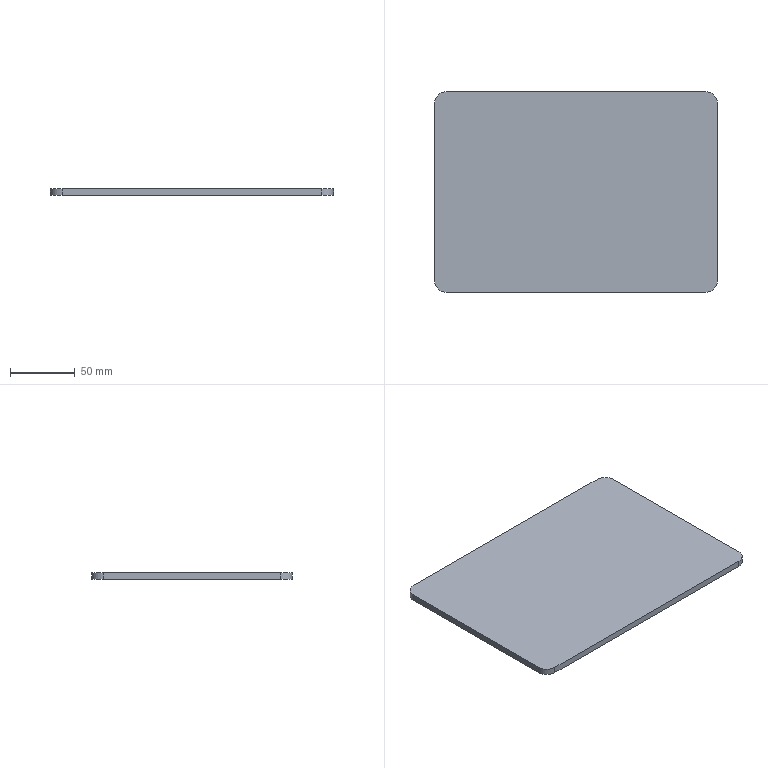Part | SolidWorks | features Extrusion 1, Fillet 1 | 1 solid | 10 faces | box 219 x 155 x 5 mm | volume 169377 mm3 | plane 6 | cylinder 4 | commonest cylinder face diameters 18 x4
STEP:
#1=CARTESIAN_POINT('',(0.,-9.,0.));
#2=VERTEX_POINT('',#1);
#3=CARTESIAN_POINT('',(0.,-146.,0.));
#4=VERTEX_POINT('',#3);
#5=CARTESIAN_POINT('',(0.,0.,0.));
#6=DIRECTION('',(0.,-1.,0.));
#7=VECTOR('',#6,1000.);
#8=LINE('',#5,#7);
#9=EDGE_CURVE('',#2,#4,#8,.T.);
#10=ORIENTED_EDGE('',*,*,#9,.T.);
#11=CARTESIAN_POINT('',(0.,-146.,5.));
#12=VERTEX_POINT('',#11);
#13=CARTESIAN_POINT('',(0.,-146.,5.));
#14=DIRECTION('',(0.,0.,1.));
#15=VECTOR('',#14,1000.);
#16=LINE('',#13,#15);
#17=EDGE_CURVE('',#4,#12,#16,.T.);
#18=ORIENTED_EDGE('',*,*,#17,.T.);
#19=CARTESIAN_POINT('',(0.,-9.,5.));
#20=VERTEX_POINT('',#19);
#21=CARTESIAN_POINT('',(0.,0.,5.));
#22=DIRECTION('',(0.,-1.,0.));
#23=VECTOR('',#22,1000.);
#24=LINE('',#21,#23);
#25=EDGE_CURVE('',#20,#12,#24,.T.);
#26=ORIENTED_EDGE('',*,*,#25,.F.);
#27=CARTESIAN_POINT('',(0.,-9.,5.));
#28=DIRECTION('',(0.,0.,-1.));
#29=VECTOR('',#28,1000.);
#30=LINE('',#27,#29);
#31=EDGE_CURVE('',#20,#2,#30,.T.);
#32=ORIENTED_EDGE('',*,*,#31,.T.);
#33=EDGE_LOOP('',(#10,#18,#26,#32));
#34=FACE_OUTER_BOUND('',#33,.T.);
#35=CARTESIAN_POINT('',(0.,0.,5.));
#36=DIRECTION('',(1.,0.,0.));
#37=DIRECTION('',(0.,1.,0.));
#38=AXIS2_PLACEMENT_3D('',#35,#36,#37);
#39=PLANE('',#38);
#40=ADVANCED_FACE('',(#34),#39,.F.);
#41=CARTESIAN_POINT('',(9.,-155.,0.));
#42=VERTEX_POINT('',#41);
#43=CARTESIAN_POINT('',(210.,-155.,0.));
#44=VERTEX_POINT('',#43);
#45=CARTESIAN_POINT('',(0.,-155.,0.));
#46=DIRECTION('',(1.,0.,0.));
#47=VECTOR('',#46,1000.);
#48=LINE('',#45,#47);
#49=EDGE_CURVE('',#42,#44,#48,.T.);
#50=ORIENTED_EDGE('',*,*,#49,.T.);
#51=CARTESIAN_POINT('',(210.,-155.,5.));
#52=VERTEX_POINT('',#51);
#53=CARTESIAN_POINT('',(210.,-155.,5.));
#54=DIRECTION('',(0.,0.,1.));
#55=VECTOR('',#54,1000.);
#56=LINE('',#53,#55);
#57=EDGE_CURVE('',#44,#52,#56,.T.);
#58=ORIENTED_EDGE('',*,*,#57,.T.);
#59=CARTESIAN_POINT('',(9.,-155.,5.));
#60=VERTEX_POINT('',#59);
#61=CARTESIAN_POINT('',(0.,-155.,5.));
#62=DIRECTION('',(1.,0.,0.));
#63=VECTOR('',#62,1000.);
#64=LINE('',#61,#63);
#65=EDGE_CURVE('',#60,#52,#64,.T.);
#66=ORIENTED_EDGE('',*,*,#65,.F.);
#67=CARTESIAN_POINT('',(9.,-155.,5.));
#68=DIRECTION('',(0.,0.,-1.));
#69=VECTOR('',#68,1000.);
#70=LINE('',#67,#69);
#71=EDGE_CURVE('',#60,#42,#70,.T.);
#72=ORIENTED_EDGE('',*,*,#71,.T.);
#73=EDGE_LOOP('',(#50,#58,#66,#72));
#74=FACE_OUTER_BOUND('',#73,.T.);
#75=CARTESIAN_POINT('',(0.,-155.,5.));
#76=DIRECTION('',(0.,1.,0.));
#77=DIRECTION('',(0.,0.,1.));
#78=AXIS2_PLACEMENT_3D('',#75,#76,#77);
#79=PLANE('',#78);
#80=ADVANCED_FACE('',(#74),#79,.F.);
#81=CARTESIAN_POINT('',(219.,-146.,0.));
#82=VERTEX_POINT('',#81);
#83=CARTESIAN_POINT('',(219.,-9.,0.));
#84=VERTEX_POINT('',#83);
#85=CARTESIAN_POINT('',(219.,0.,0.));
#86=DIRECTION('',(0.,1.,0.));
#87=VECTOR('',#86,1000.);
#88=LINE('',#85,#87);
#89=EDGE_CURVE('',#82,#84,#88,.T.);
#90=ORIENTED_EDGE('',*,*,#89,.T.);
#91=CARTESIAN_POINT('',(219.,-9.,5.));
#92=VERTEX_POINT('',#91);
#93=CARTESIAN_POINT('',(219.,-9.,5.));
#94=DIRECTION('',(0.,0.,1.));
#95=VECTOR('',#94,1000.);
#96=LINE('',#93,#95);
#97=EDGE_CURVE('',#84,#92,#96,.T.);
#98=ORIENTED_EDGE('',*,*,#97,.T.);
#99=CARTESIAN_POINT('',(219.,-146.,5.));
#100=VERTEX_POINT('',#99);
#101=CARTESIAN_POINT('',(219.,0.,5.));
#102=DIRECTION('',(0.,1.,0.));
#103=VECTOR('',#102,1000.);
#104=LINE('',#101,#103);
#105=EDGE_CURVE('',#100,#92,#104,.T.);
#106=ORIENTED_EDGE('',*,*,#105,.F.);
#107=CARTESIAN_POINT('',(219.,-146.,5.));
#108=DIRECTION('',(0.,0.,-1.));
#109=VECTOR('',#108,1000.);
#110=LINE('',#107,#109);
#111=EDGE_CURVE('',#100,#82,#110,.T.);
#112=ORIENTED_EDGE('',*,*,#111,.T.);
#113=EDGE_LOOP('',(#90,#98,#106,#112));
#114=FACE_OUTER_BOUND('',#113,.T.);
#115=CARTESIAN_POINT('',(219.,0.,5.));
#116=DIRECTION('',(-1.,0.,0.));
#117=DIRECTION('',(0.,-1.,0.));
#118=AXIS2_PLACEMENT_3D('',#115,#116,#117);
#119=PLANE('',#118);
#120=ADVANCED_FACE('',(#114),#119,.F.);
#121=CARTESIAN_POINT('',(210.,0.,5.));
#122=VERTEX_POINT('',#121);
#123=CARTESIAN_POINT('',(9.,0.,5.));
#124=VERTEX_POINT('',#123);
#125=CARTESIAN_POINT('',(0.,0.,5.));
#126=DIRECTION('',(-1.,0.,0.));
#127=VECTOR('',#126,1000.);
#128=LINE('',#125,#127);
#129=EDGE_CURVE('',#122,#124,#128,.T.);
#130=ORIENTED_EDGE('',*,*,#129,.F.);
#131=CARTESIAN_POINT('',(210.,0.,0.));
#132=VERTEX_POINT('',#131);
#133=CARTESIAN_POINT('',(210.,0.,5.));
#134=DIRECTION('',(0.,0.,-1.));
#135=VECTOR('',#134,1000.);
#136=LINE('',#133,#135);
#137=EDGE_CURVE('',#122,#132,#136,.T.);
#138=ORIENTED_EDGE('',*,*,#137,.T.);
#139=CARTESIAN_POINT('',(9.,0.,0.));
#140=VERTEX_POINT('',#139);
#141=CARTESIAN_POINT('',(0.,0.,0.));
#142=DIRECTION('',(-1.,0.,0.));
#143=VECTOR('',#142,1000.);
#144=LINE('',#141,#143);
#145=EDGE_CURVE('',#132,#140,#144,.T.);
#146=ORIENTED_EDGE('',*,*,#145,.T.);
#147=CARTESIAN_POINT('',(9.,0.,5.));
#148=DIRECTION('',(0.,0.,1.));
#149=VECTOR('',#148,1000.);
#150=LINE('',#147,#149);
#151=EDGE_CURVE('',#140,#124,#150,.T.);
#152=ORIENTED_EDGE('',*,*,#151,.T.);
#153=EDGE_LOOP('',(#130,#138,#146,#152));
#154=FACE_OUTER_BOUND('',#153,.T.);
#155=CARTESIAN_POINT('',(0.,0.,5.));
#156=DIRECTION('',(0.,-1.,0.));
#157=DIRECTION('',(0.,0.,-1.));
#158=AXIS2_PLACEMENT_3D('',#155,#156,#157);
#159=PLANE('',#158);
#160=ADVANCED_FACE('',(#154),#159,.F.);
#161=ORIENTED_EDGE('',*,*,#105,.T.);
#162=CARTESIAN_POINT('',(210.,-9.,5.));
#163=DIRECTION('',(0.,0.,1.));
#164=DIRECTION('',(1.,0.,0.));
#165=AXIS2_PLACEMENT_3D('',#162,#163,#164);
#166=CIRCLE('',#165,9.);
#167=EDGE_CURVE('',#92,#122,#166,.T.);
#168=ORIENTED_EDGE('',*,*,#167,.T.);
#169=ORIENTED_EDGE('',*,*,#129,.T.);
#170=CARTESIAN_POINT('',(9.,-9.,5.));
#171=DIRECTION('',(0.,0.,1.));
#172=DIRECTION('',(1.,0.,0.));
#173=AXIS2_PLACEMENT_3D('',#170,#171,#172);
#174=CIRCLE('',#173,9.);
#175=EDGE_CURVE('',#124,#20,#174,.T.);
#176=ORIENTED_EDGE('',*,*,#175,.T.);
#177=ORIENTED_EDGE('',*,*,#25,.T.);
#178=CARTESIAN_POINT('',(9.,-146.,5.));
#179=DIRECTION('',(0.,0.,1.));
#180=DIRECTION('',(1.,0.,0.));
#181=AXIS2_PLACEMENT_3D('',#178,#179,#180);
#182=CIRCLE('',#181,9.);
#183=EDGE_CURVE('',#12,#60,#182,.T.);
#184=ORIENTED_EDGE('',*,*,#183,.T.);
#185=ORIENTED_EDGE('',*,*,#65,.T.);
#186=CARTESIAN_POINT('',(210.,-146.,5.));
#187=DIRECTION('',(0.,0.,1.));
#188=DIRECTION('',(1.,0.,0.));
#189=AXIS2_PLACEMENT_3D('',#186,#187,#188);
#190=CIRCLE('',#189,9.);
#191=EDGE_CURVE('',#52,#100,#190,.T.);
#192=ORIENTED_EDGE('',*,*,#191,.T.);
#193=EDGE_LOOP('',(#161,#168,#169,#176,#177,#184,#185,#192));
#194=FACE_OUTER_BOUND('',#193,.T.);
#195=CARTESIAN_POINT('',(0.,0.,5.));
#196=DIRECTION('',(0.,0.,1.));
#197=DIRECTION('',(1.,0.,0.));
#198=AXIS2_PLACEMENT_3D('',#195,#196,#197);
#199=PLANE('',#198);
#200=ADVANCED_FACE('',(#194),#199,.T.);
#201=ORIENTED_EDGE('',*,*,#145,.F.);
#202=CARTESIAN_POINT('',(210.,-9.,0.));
#203=DIRECTION('',(0.,0.,-1.));
#204=DIRECTION('',(1.,0.,0.));
#205=AXIS2_PLACEMENT_3D('',#202,#203,#204);
#206=CIRCLE('',#205,9.);
#207=EDGE_CURVE('',#132,#84,#206,.T.);
#208=ORIENTED_EDGE('',*,*,#207,.T.);
#209=ORIENTED_EDGE('',*,*,#89,.F.);
#210=CARTESIAN_POINT('',(210.,-146.,0.));
#211=DIRECTION('',(0.,0.,-1.));
#212=DIRECTION('',(1.,0.,0.));
#213=AXIS2_PLACEMENT_3D('',#210,#211,#212);
#214=CIRCLE('',#213,9.);
#215=EDGE_CURVE('',#82,#44,#214,.T.);
#216=ORIENTED_EDGE('',*,*,#215,.T.);
#217=ORIENTED_EDGE('',*,*,#49,.F.);
#218=CARTESIAN_POINT('',(9.,-146.,0.));
#219=DIRECTION('',(0.,0.,-1.));
#220=DIRECTION('',(1.,0.,0.));
#221=AXIS2_PLACEMENT_3D('',#218,#219,#220);
#222=CIRCLE('',#221,9.);
#223=EDGE_CURVE('',#42,#4,#222,.T.);
#224=ORIENTED_EDGE('',*,*,#223,.T.);
#225=ORIENTED_EDGE('',*,*,#9,.F.);
#226=CARTESIAN_POINT('',(9.,-9.,0.));
#227=DIRECTION('',(0.,0.,-1.));
#228=DIRECTION('',(1.,0.,0.));
#229=AXIS2_PLACEMENT_3D('',#226,#227,#228);
#230=CIRCLE('',#229,9.);
#231=EDGE_CURVE('',#2,#140,#230,.T.);
#232=ORIENTED_EDGE('',*,*,#231,.T.);
#233=EDGE_LOOP('',(#201,#208,#209,#216,#217,#224,#225,#232));
#234=FACE_OUTER_BOUND('',#233,.T.);
#235=CARTESIAN_POINT('',(0.,0.,0.));
#236=DIRECTION('',(0.,0.,1.));
#237=DIRECTION('',(1.,0.,0.));
#238=AXIS2_PLACEMENT_3D('',#235,#236,#237);
#239=PLANE('',#238);
#240=ADVANCED_FACE('',(#234),#239,.F.);
#241=ORIENTED_EDGE('',*,*,#167,.F.);
#242=ORIENTED_EDGE('',*,*,#97,.F.);
#243=ORIENTED_EDGE('',*,*,#207,.F.);
#244=ORIENTED_EDGE('',*,*,#137,.F.);
#245=EDGE_LOOP('',(#241,#242,#243,#244));
#246=FACE_OUTER_BOUND('',#245,.T.);
#247=CARTESIAN_POINT('',(210.,-9.,5.));
#248=DIRECTION('',(0.,0.,-1.));
#249=DIRECTION('',(-1.,0.,0.));
#250=AXIS2_PLACEMENT_3D('',#247,#248,#249);
#251=CYLINDRICAL_SURFACE('',#250,9.);
#252=ADVANCED_FACE('',(#246),#251,.T.);
#253=ORIENTED_EDGE('',*,*,#191,.F.);
#254=ORIENTED_EDGE('',*,*,#57,.F.);
#255=ORIENTED_EDGE('',*,*,#215,.F.);
#256=ORIENTED_EDGE('',*,*,#111,.F.);
#257=EDGE_LOOP('',(#253,#254,#255,#256));
#258=FACE_OUTER_BOUND('',#257,.T.);
#259=CARTESIAN_POINT('',(210.,-146.,5.));
#260=DIRECTION('',(0.,0.,-1.));
#261=DIRECTION('',(-1.,0.,0.));
#262=AXIS2_PLACEMENT_3D('',#259,#260,#261);
#263=CYLINDRICAL_SURFACE('',#262,9.);
#264=ADVANCED_FACE('',(#258),#263,.T.);
#265=ORIENTED_EDGE('',*,*,#183,.F.);
#266=ORIENTED_EDGE('',*,*,#17,.F.);
#267=ORIENTED_EDGE('',*,*,#223,.F.);
#268=ORIENTED_EDGE('',*,*,#71,.F.);
#269=EDGE_LOOP('',(#265,#266,#267,#268));
#270=FACE_OUTER_BOUND('',#269,.T.);
#271=CARTESIAN_POINT('',(9.,-146.,5.));
#272=DIRECTION('',(0.,0.,-1.));
#273=DIRECTION('',(-1.,0.,0.));
#274=AXIS2_PLACEMENT_3D('',#271,#272,#273);
#275=CYLINDRICAL_SURFACE('',#274,9.);
#276=ADVANCED_FACE('',(#270),#275,.T.);
#277=ORIENTED_EDGE('',*,*,#175,.F.);
#278=ORIENTED_EDGE('',*,*,#151,.F.);
#279=ORIENTED_EDGE('',*,*,#231,.F.);
#280=ORIENTED_EDGE('',*,*,#31,.F.);
#281=EDGE_LOOP('',(#277,#278,#279,#280));
#282=FACE_OUTER_BOUND('',#281,.T.);
#283=CARTESIAN_POINT('',(9.,-9.,5.));
#284=DIRECTION('',(0.,0.,-1.));
#285=DIRECTION('',(-1.,0.,0.));
#286=AXIS2_PLACEMENT_3D('',#283,#284,#285);
#287=CYLINDRICAL_SURFACE('',#286,9.);
#288=ADVANCED_FACE('',(#282),#287,.T.);
#289=CLOSED_SHELL('',(#40,#80,#120,#160,#200,#240,#252,#264,#276,#288));
#290=MANIFOLD_SOLID_BREP('',#289);
#291=CARTESIAN_POINT('',(0.,0.,0.));
#292=DIRECTION('',(0.,0.,1.));
#293=DIRECTION('',(1.,0.,0.));
#294=AXIS2_PLACEMENT_3D('',#291,#292,#293);
#295=(LENGTH_UNIT()NAMED_UNIT(*)SI_UNIT(.MILLI.,.METRE.));
#296=UNCERTAINTY_MEASURE_WITH_UNIT(LENGTH_MEASURE(0.00001),#295,'','');
#297=(NAMED_UNIT(*)PLANE_ANGLE_UNIT()SI_UNIT($,.RADIAN.));
#298=(NAMED_UNIT(*)SI_UNIT($,.STERADIAN.)SOLID_ANGLE_UNIT());
#299=(GEOMETRIC_REPRESENTATION_CONTEXT(3)GLOBAL_UNCERTAINTY_ASSIGNED_CONTEXT((#296))GLOBAL_UNIT_ASSIGNED_CONTEXT((#295,#297,#298))REPRESENTATION_CONTEXT('',''));
#300=ADVANCED_BREP_SHAPE_REPRESENTATION('',(#290,#294),#299);